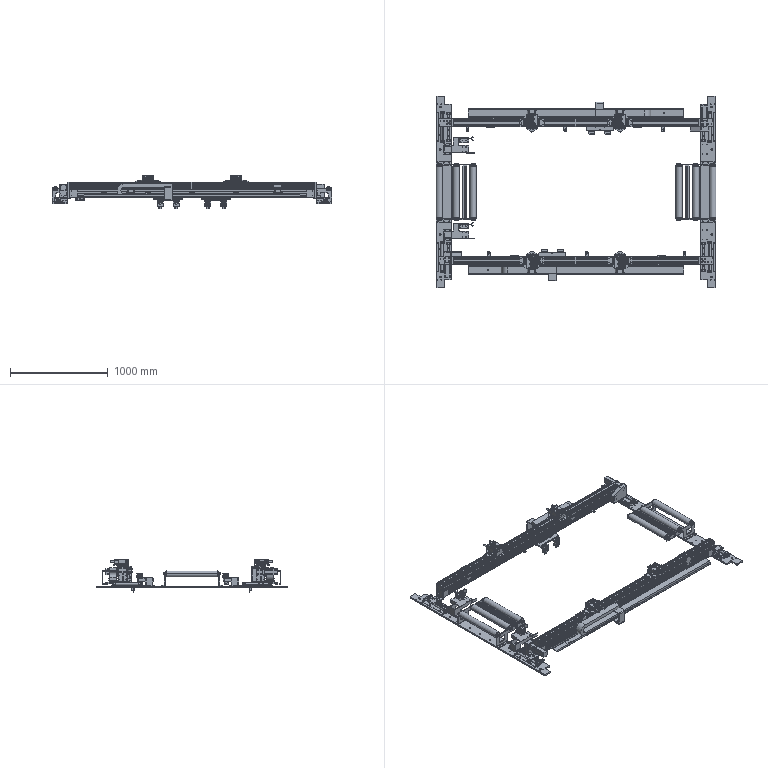Part | SolidWorks | 232 solids | 12544 faces | volume 84353797 mm3 | plane 5564 | cylinder 4954 | cone 1172 | torus 496 | sphere 256 | spline 102 | commonest cylinder face diameters 9 x412 5 x278 7 x272 6.8 x264 0.4 x256 4 x228